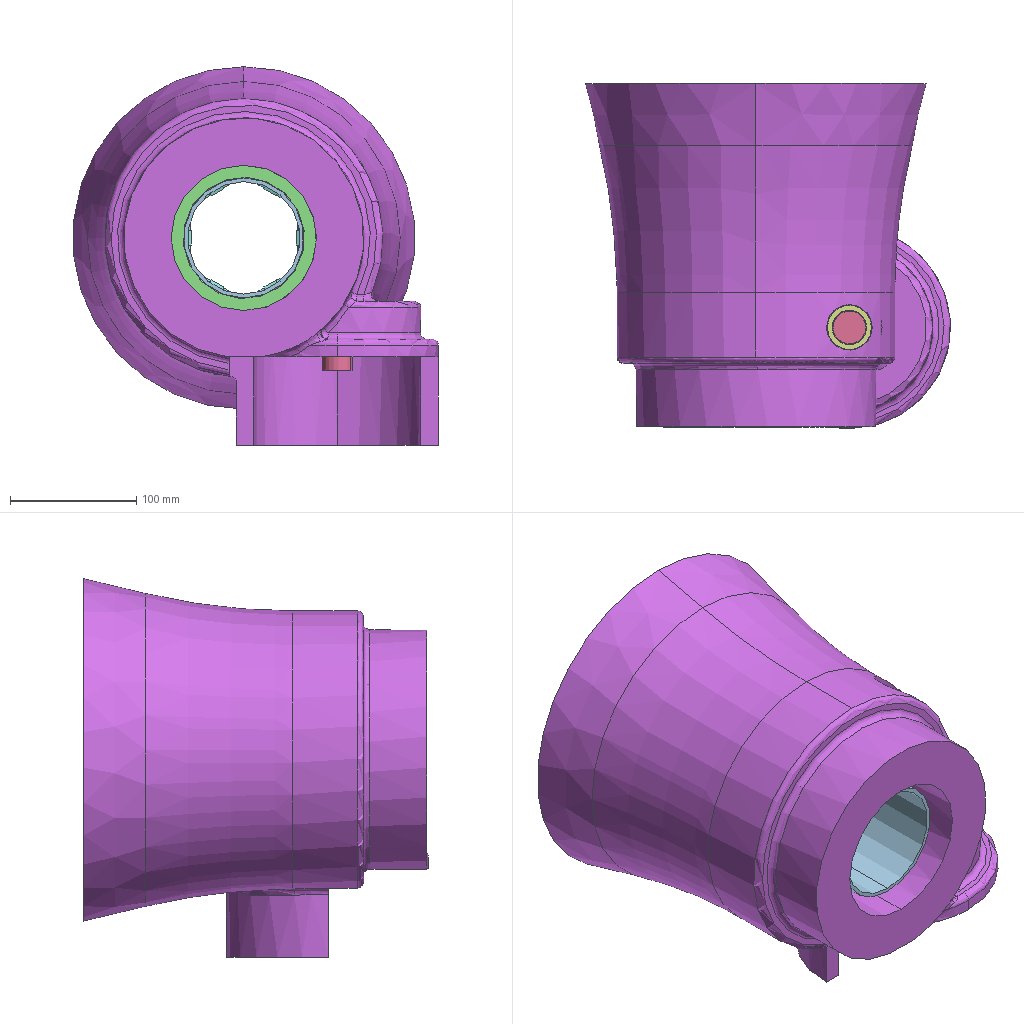Assembly | SolidWorks | 13 different items | 62 placed | box 289 x 273 x 299 mm
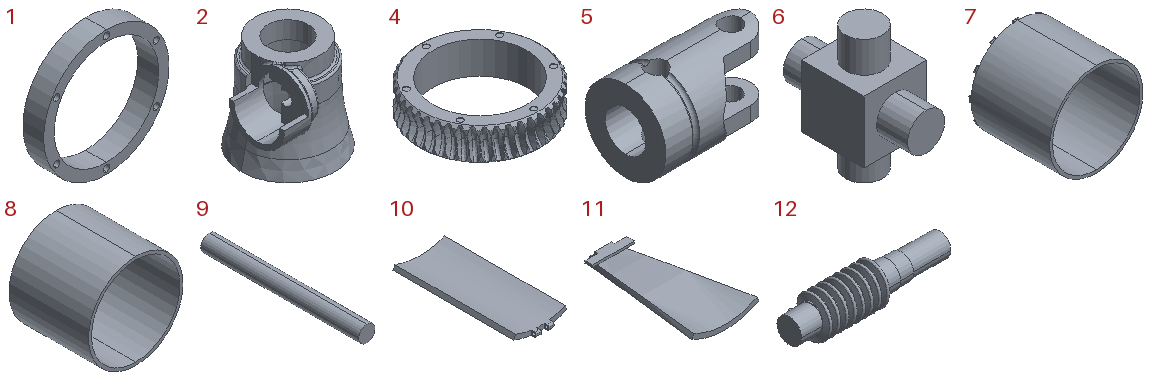Parts list (item | name | quantity | size | volume | features):
1 | - | x1 | 120 x 20 x 120 mm | 65722 mm3 | features CirPattern 1, Extrusion 1, ICE 1
2 | - | x1 | 299.386 x 289.264 x 272.746 mm | 5989690 mm3 | features Cut 4, Fillet 4, ICE 4, Extrusion 1, Revolution 1
3 | - | x1 | - | - | -
4 | - | x1 | 125.684 x 125.684 x 32.802 mm | 115806 mm3 | features CirPattern 2, Helix 2, ICE 2, SweepCut 2, Chamfer 1, Extrusion 1, RevCut 1, Scale 1
5 | - | x24 | 18.5 x 12 x 12 mm | 994.075 mm3 | features ICE 2, RefPoint 1, Revolution 1
6 | - | x12 | 5 x 10 x 10 mm | 195.686 mm3 | features ICE 2, Extrusion 1
7 | - | x1 | 95 x 83 x 95 mm | 69660 mm3 | features CirPattern 1, Extrusion 1, ICE 1
8 | - | x1 | 95 x 80 x 95 mm | 69366 mm3 | features Extrusion 1
9 | - | x6 | 6 x 58 x 6 mm | 1640 mm3 | features Extrusion 1
10 | - | x6 | 35.207 x 83 x 6.273 mm | 8409 mm3 | features ICE 3, Blend 1, Fillet 1
11 | - | x6 | 43.809 x 83 x 8.178 mm | 7265 mm3 | features ICE 6, MoveFace 6, Blend 1, Fillet 1
12 | - | x1 | 158.95 x 40.46 x 40.46 mm | 106297 mm3 | features Helix 2, Sweep 2, ICE 1, Revolution 1, Scale 1
13 | Motor | x1 | - | - | -
Mates (type | each side: item.copy, entity, surface, feature):
Concentric | 7.1 face cylinder Boss-Extrude 1 | 1.1 face cylinder Boss-Extrude 1
Concentric | 7.1 face cylinder CirPattern 1 | 11.1 face cylinder Cut-Extrude 1
Coincident | 7.1 face plane CirPattern 1 | 11.1 face plane Boss-Extrude 4
Concentric | 7.1 face cylinder Boss-Extrude 3 | 10.1 face cylinder Cut-Extrude 2
Coincident | 7.1 face plane Boss-Extrude 3 | 10.1 face plane Boss-Extrude 1
Coincident | 10.1 face cylinder Loft1 | 11.1 vertex
Concentric | 10.1 face cylinder Cut-Extrude 3 | 5.1 face cylinder Cut-Extrude 1
Tangent | 10.1 face cylinder Loft1 | 5.1 face cylinder Revolve 3
Concentric | 6.1 face cylinder Boss-Extrude 3 | 5.1 face cylinder Cut-Extrude 1
Concentric | 5.2 face cylinder Cut-Extrude 1 | 6.1 face cylinder Boss-Extrude 2
Coincident | 6.1 select_type:25 | 5.1 point
Coincident | 5.2 point | 6.1 select_type:25
Coincident | 1.1 face plane Boss-Extrude 1 | 5.3 face plane Revolve 3
Concentric | 1.1 face cylinder CirPattern 1 | 5.3 face cylinder Revolve 3
Concentric | 6.2 face cylinder Boss-Extrude 3 | 5.3 face cylinder Cut-Extrude 1
Concentric | 5.4 face cylinder Cut-Extrude 1 | 6.2 face cylinder Boss-Extrude 2
Coincident | 5.4 point | 6.2 select_type:25
Coincident | 6.2 select_type:25 | 5.3 point
Concentric | 5.2 face cylinder Revolve 3 | 5.4 face cylinder Revolve 3
Concentric | 5.2 face cylinder Revolve 3 | assembly face
Concentric | 5.4 face cylinder Revolve 3 | assembly face
Coincident | 5.4 face plane Revolve 3 | assembly face
Concentric | 9.1 face cylinder Boss-Extrude 1 | 5.4 face cylinder Revolve 3
Concentric | 9.1 face cylinder Boss-Extrude 1 | 5.2 face cylinder Revolve 3
Coincident | 9.1 face plane Boss-Extrude 1 | 5.4 face plane Revolve 3
Coincident | 9.1 face plane Boss-Extrude 1 | 5.2 face plane Revolve 3
Coincident | 7.1 face plane Boss-Extrude 1 | 1.1 face plane Boss-Extrude 1
Concentric | 1.1 face cylinder Boss-Extrude 1 | 4.1 face cylinder Cut-Extrude 3
Concentric | 1.1 face cylinder Cut-Extrude 1 | 4.1 face cylinder CirPattern 1
Coincident | 1.1 face plane Boss-Extrude 1 | 4.1 face plane Boss-Extrude1
Coincident | 4.1 plane | 12.1 axis
GearDim | 12.1 face cylinder Revolve1 | 4.1 edge
Parallel | 7.1 plane | 12.1 face plane Revolve1
DistanceDim | 7.1 plane | 12.1 axis
DistanceDim | 12.1 face plane Revolve1 | 7.1 plane
Coincident | 7.1 face plane Boss-Extrude 1 | 8.1 face plane Boss-Extrude 1
Concentric | 7.1 face cylinder Boss-Extrude 1 | 8.1 face cylinder Boss-Extrude 1
InPlace | 12.1 face plane Revolve1 | 3.1 plane
Concentric | 8.1 face cylinder Boss-Extrude 1 | 2.1 face cylinder Boss-Extrude 1
DistanceDim | 8.1 face plane Boss-Extrude 1 | 2.1 face plane Boss-Extrude 1
Parallel | 2.1 plane | assembly plane